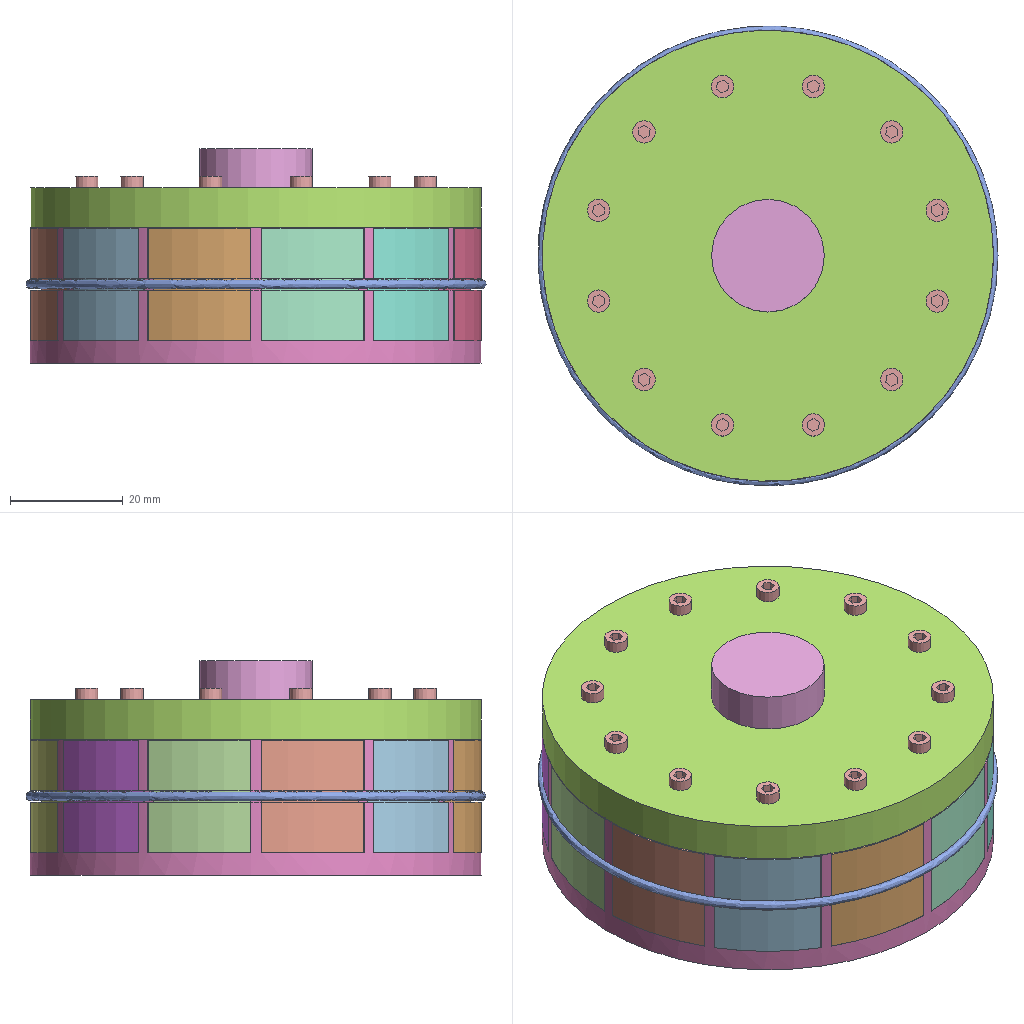Assembly | NX | 6 different items | 17 placed | box 82 x 82 x 38 mm
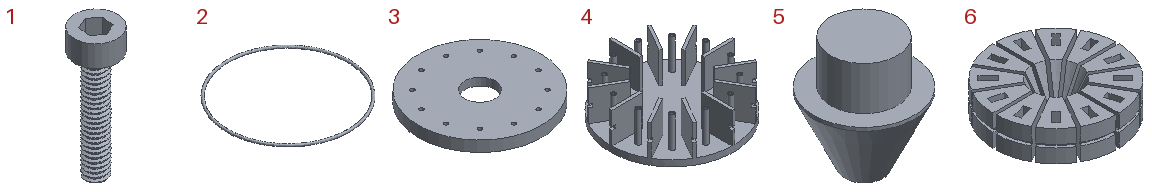Parts list (item | quantity | size | volume | features):
1 | x12 | 4 x 4 x 12 mm | 45.055 mm3 | features DATUM_CSYS 4, EXTRUDE 3, SKETCH 3, THREADS 1
2 | x1 | 81.599 x 81.597 x 1.6 mm | 504.996 mm3 | features DATUM_CSYS 3, SKETCH 2, SKIN 1
3 | x1 | 80 x 80 x 7 mm | 31789 mm3 | features DATUM_CSYS 7, EXTRUDE 7, SKETCH 6, REPLACE_FACE 1
4 | x1 | 80 x 80 x 24.1 mm | 26700 mm3 | features SIMPLE HOLE 12, SYMBOLIC_THREAD 12, DATUM_CSYS 7, EXTRUDE 6, SKETCH 6, HOLE PACKAGE 1, SWP104 1
5 | x1 | 30 x 30 x 34 mm | 11960 mm3 | features DATUM_CSYS 3, SKETCH 2, EXTRUDE 1, SWP104 1
6 | x1 | 79.975 x 79.975 x 19.9 mm | 69186 mm3 | features SUBTRACT 12, DATUM_CSYS 4, SKETCH 3, EXTRUDE 2, OFFSET_REGION 1, SWP104 1
Mates (type | each side: item.copy, entity, surface, feature):
Fix | 4.1 component
Touch | 3.1 face plane Extrude(1) | 4.1 face plane Extrude(4)